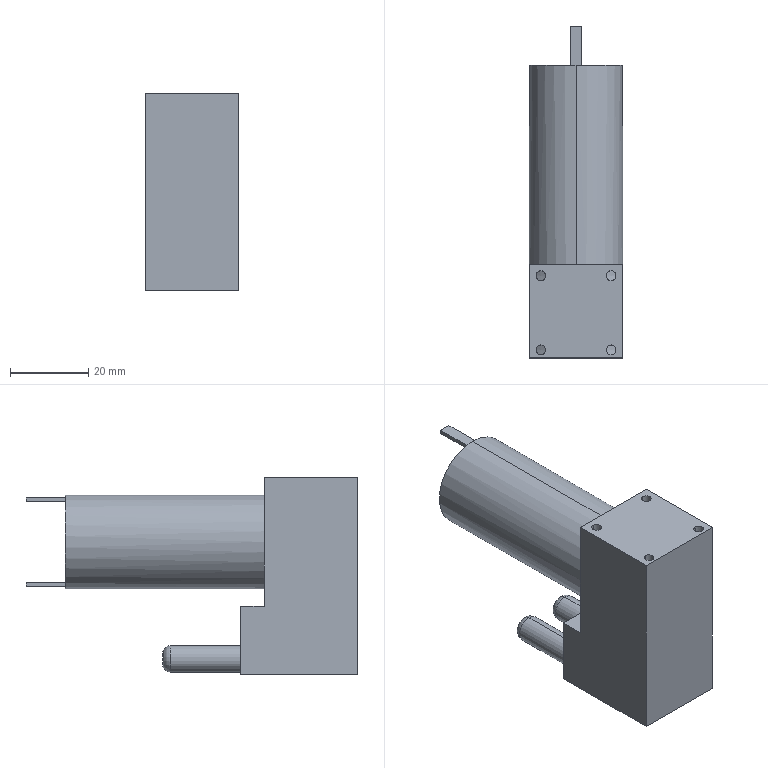Part | SolidWorks | features BaseBody 1 | 1 solid | 44 faces | box 24 x 85 x 50.5 mm | volume 56047 mm3 | plane 22 | cylinder 14 | torus 4 | cone 4 | commonest cylinder face diameters 2.5 x8 6.8 x4 24 x2